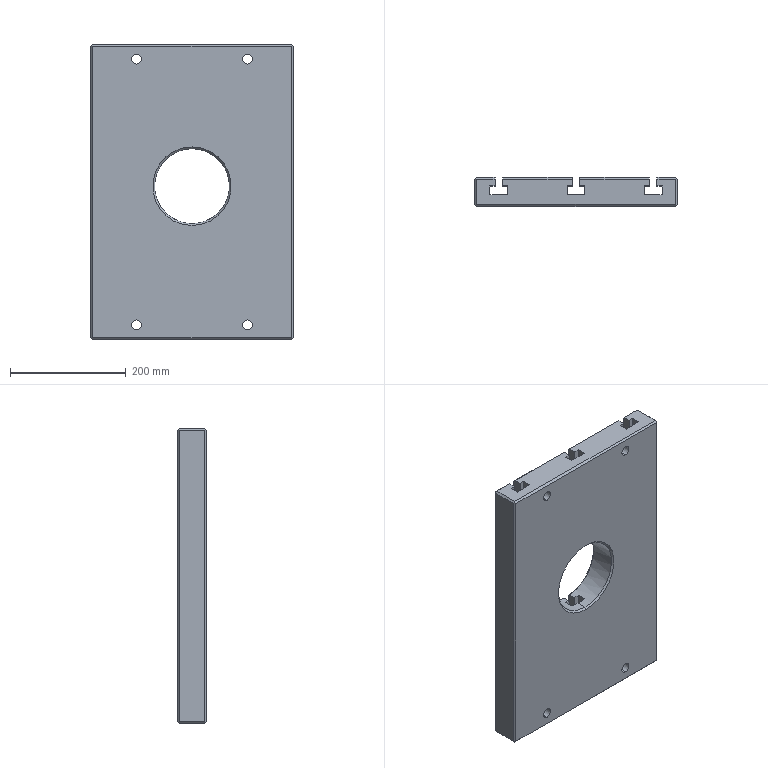Part | Creo | features CURVE 3, DATUM PLANE 3, CUT 2, CHAMFER 1, COORDINATE SYSTEM 1, PROTRUSION 1 | 1 solid | 81 faces | box 349.97 x 50 x 510 mm | volume 7245809 mm3 | plane 59 | cylinder 18 | cone 4 | commonest cylinder face diameters 17 x8 27.784 x8 130 x2